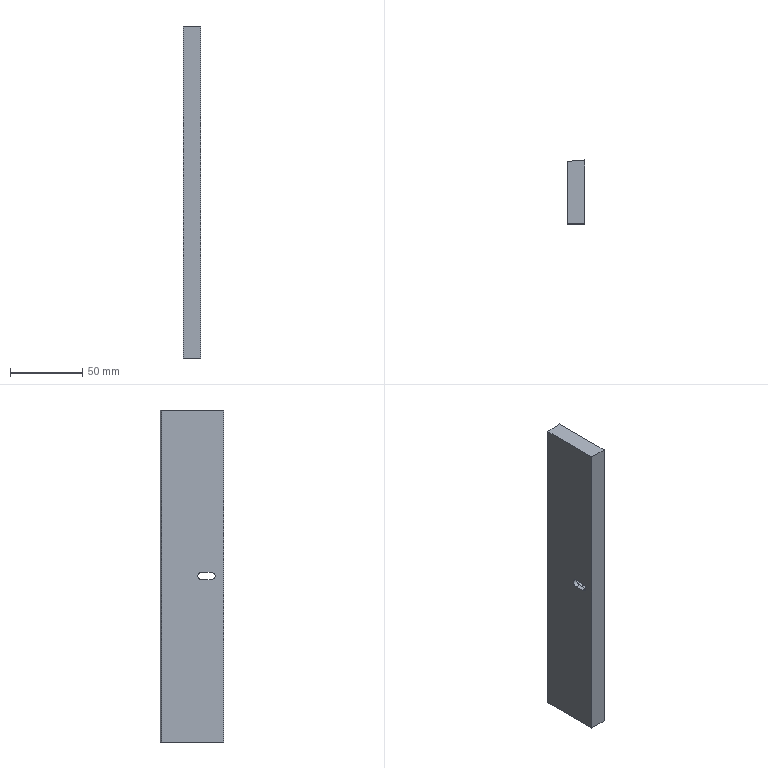Part | STEP file | A14-028 | 1 solid | 15 faces | box 12 x 44 x 230 mm | volume 118590 mm3 | plane 11 | cylinder 4 | commonest cylinder face diameters 5.5 x2 10 x2
STEP:
#1=CARTESIAN_POINT('',(0.,0.,0.));
#2=DIRECTION('',(0.,0.,1.));
#3=DIRECTION('',(1.,0.,0.));
#4=AXIS2_PLACEMENT_3D('',#1,#2,#3);
#5=CARTESIAN_POINT('',(-6.,21.,-115.));
#6=VERTEX_POINT('',#5);
#7=CARTESIAN_POINT('',(-6.,-22.,-115.));
#8=VERTEX_POINT('',#7);
#9=CARTESIAN_POINT('',(-6.,-22.,-115.));
#10=DIRECTION('',(0.,-1.,0.));
#11=VECTOR('',#10,1.);
#12=LINE('',#9,#11);
#13=CARTESIAN_POINT('',(-6.,-22.,115.));
#14=DIRECTION('',(1.,0.,0.));
#15=DIRECTION('',(0.,1.,0.));
#16=AXIS2_PLACEMENT_3D('',#13,#14,#15);
#17=PLANE('',#16);
#18=CARTESIAN_POINT('',(0.,-230.));
#19=DIRECTION('',(-1.,0.));
#20=VECTOR('',#19,1.);
#21=LINE('',#18,#20);
#22=(GEOMETRIC_REPRESENTATION_CONTEXT(2)PARAMETRIC_REPRESENTATION_CONTEXT()REPRESENTATION_CONTEXT('',''));
#23=DEFINITIONAL_REPRESENTATION('',(#21),#22);
#24=PCURVE('',#17,#23);
#25=CARTESIAN_POINT('',(0.,0.,-115.));
#26=DIRECTION('',(0.,0.,1.));
#27=DIRECTION('',(1.,0.,0.));
#28=AXIS2_PLACEMENT_3D('',#25,#26,#27);
#29=PLANE('',#28);
#30=CARTESIAN_POINT('',(-6.,-22.));
#31=DIRECTION('',(0.,-1.));
#32=VECTOR('',#31,1.);
#33=LINE('',#30,#32);
#34=(GEOMETRIC_REPRESENTATION_CONTEXT(2)PARAMETRIC_REPRESENTATION_CONTEXT()REPRESENTATION_CONTEXT('',''));
#35=DEFINITIONAL_REPRESENTATION('',(#33),#34);
#36=PCURVE('',#29,#35);
#37=SURFACE_CURVE('',#12,(#24,#36),.PCURVE_S1.);
#38=EDGE_CURVE('',#6,#8,#37,.T.);
#39=ORIENTED_EDGE('',*,*,#38,.T.);
#40=CARTESIAN_POINT('',(-6.,-22.,115.));
#41=VERTEX_POINT('',#40);
#42=CARTESIAN_POINT('',(-6.,-22.,115.));
#43=DIRECTION('',(0.,0.,-1.));
#44=VECTOR('',#43,1.);
#45=LINE('',#42,#44);
#46=CARTESIAN_POINT('',(0.,0.));
#47=DIRECTION('',(0.,-1.));
#48=VECTOR('',#47,1.);
#49=LINE('',#46,#48);
#50=(GEOMETRIC_REPRESENTATION_CONTEXT(2)PARAMETRIC_REPRESENTATION_CONTEXT()REPRESENTATION_CONTEXT('',''));
#51=DEFINITIONAL_REPRESENTATION('',(#49),#50);
#52=PCURVE('',#17,#51);
#53=CARTESIAN_POINT('',(6.,-22.,115.));
#54=DIRECTION('',(0.,1.,0.));
#55=DIRECTION('',(0.,0.,1.));
#56=AXIS2_PLACEMENT_3D('',#53,#54,#55);
#57=PLANE('',#56);
#58=CARTESIAN_POINT('',(0.,-12.));
#59=DIRECTION('',(-1.,0.));
#60=VECTOR('',#59,1.);
#61=LINE('',#58,#60);
#62=(GEOMETRIC_REPRESENTATION_CONTEXT(2)PARAMETRIC_REPRESENTATION_CONTEXT()REPRESENTATION_CONTEXT('',''));
#63=DEFINITIONAL_REPRESENTATION('',(#61),#62);
#64=PCURVE('',#57,#63);
#65=SURFACE_CURVE('',#45,(#52,#64),.PCURVE_S1.);
#66=EDGE_CURVE('',#41,#8,#65,.T.);
#67=ORIENTED_EDGE('',*,*,#66,.F.);
#68=CARTESIAN_POINT('',(-6.,21.,115.));
#69=VERTEX_POINT('',#68);
#70=CARTESIAN_POINT('',(-6.,-22.,115.));
#71=DIRECTION('',(0.,-1.,0.));
#72=VECTOR('',#71,1.);
#73=LINE('',#70,#72);
#74=CARTESIAN_POINT('',(0.,0.));
#75=DIRECTION('',(-1.,0.));
#76=VECTOR('',#75,1.);
#77=LINE('',#74,#76);
#78=(GEOMETRIC_REPRESENTATION_CONTEXT(2)PARAMETRIC_REPRESENTATION_CONTEXT()REPRESENTATION_CONTEXT('',''));
#79=DEFINITIONAL_REPRESENTATION('',(#77),#78);
#80=PCURVE('',#17,#79);
#81=CARTESIAN_POINT('',(0.,0.,115.));
#82=DIRECTION('',(0.,0.,1.));
#83=DIRECTION('',(1.,0.,0.));
#84=AXIS2_PLACEMENT_3D('',#81,#82,#83);
#85=PLANE('',#84);
#86=CARTESIAN_POINT('',(-6.,-22.));
#87=DIRECTION('',(0.,-1.));
#88=VECTOR('',#87,1.);
#89=LINE('',#86,#88);
#90=(GEOMETRIC_REPRESENTATION_CONTEXT(2)PARAMETRIC_REPRESENTATION_CONTEXT()REPRESENTATION_CONTEXT('',''));
#91=DEFINITIONAL_REPRESENTATION('',(#89),#90);
#92=PCURVE('',#85,#91);
#93=SURFACE_CURVE('',#73,(#80,#92),.PCURVE_S1.);
#94=EDGE_CURVE('',#69,#41,#93,.T.);
#95=ORIENTED_EDGE('',*,*,#94,.F.);
#96=CARTESIAN_POINT('',(-6.,21.,115.));
#97=DIRECTION('',(0.,0.,-1.));
#98=VECTOR('',#97,1.);
#99=LINE('',#96,#98);
#100=CARTESIAN_POINT('',(43.,0.));
#101=DIRECTION('',(0.,-1.));
#102=VECTOR('',#101,1.);
#103=LINE('',#100,#102);
#104=(GEOMETRIC_REPRESENTATION_CONTEXT(2)PARAMETRIC_REPRESENTATION_CONTEXT()REPRESENTATION_CONTEXT('',''));
#105=DEFINITIONAL_REPRESENTATION('',(#103),#104);
#106=PCURVE('',#17,#105);
#107=CARTESIAN_POINT('',(6.,22.,115.));
#108=DIRECTION('',(0.08305,-0.9965,0.));
#109=DIRECTION('',(0.9965,0.08305,0.));
#110=AXIS2_PLACEMENT_3D('',#107,#108,#109);
#111=PLANE('',#110);
#112=CARTESIAN_POINT('',(-12.042,0.));
#113=DIRECTION('',(0.,-1.));
#114=VECTOR('',#113,1.);
#115=LINE('',#112,#114);
#116=(GEOMETRIC_REPRESENTATION_CONTEXT(2)PARAMETRIC_REPRESENTATION_CONTEXT()REPRESENTATION_CONTEXT('',''));
#117=DEFINITIONAL_REPRESENTATION('',(#115),#116);
#118=PCURVE('',#111,#117);
#119=SURFACE_CURVE('',#99,(#106,#118),.PCURVE_S1.);
#120=EDGE_CURVE('',#69,#6,#119,.T.);
#121=ORIENTED_EDGE('',*,*,#120,.T.);
#122=EDGE_LOOP('',(#39,#67,#95,#121));
#123=FACE_BOUND('',#122,.T.);
#124=CARTESIAN_POINT('',(-6.,-13.25,2.75));
#125=VERTEX_POINT('',#124);
#126=CARTESIAN_POINT('',(-6.,-6.75,2.75));
#127=VERTEX_POINT('',#126);
#128=CARTESIAN_POINT('',(-6.,-13.25,2.75));
#129=DIRECTION('',(0.,1.,0.));
#130=VECTOR('',#129,1.);
#131=LINE('',#128,#130);
#132=CARTESIAN_POINT('',(8.75,-112.25));
#133=DIRECTION('',(1.,0.));
#134=VECTOR('',#133,1.);
#135=LINE('',#132,#134);
#136=(GEOMETRIC_REPRESENTATION_CONTEXT(2)PARAMETRIC_REPRESENTATION_CONTEXT()REPRESENTATION_CONTEXT('',''));
#137=DEFINITIONAL_REPRESENTATION('',(#135),#136);
#138=PCURVE('',#17,#137);
#139=CARTESIAN_POINT('',(6.,-13.25,2.75));
#140=DIRECTION('',(0.,0.,1.));
#141=DIRECTION('',(0.,-1.,0.));
#142=AXIS2_PLACEMENT_3D('',#139,#140,#141);
#143=PLANE('',#142);
#144=CARTESIAN_POINT('',(0.,-12.));
#145=DIRECTION('',(-1.,0.));
#146=VECTOR('',#145,1.);
#147=LINE('',#144,#146);
#148=(GEOMETRIC_REPRESENTATION_CONTEXT(2)PARAMETRIC_REPRESENTATION_CONTEXT()REPRESENTATION_CONTEXT('',''));
#149=DEFINITIONAL_REPRESENTATION('',(#147),#148);
#150=PCURVE('',#143,#149);
#151=SURFACE_CURVE('',#131,(#138,#150),.PCURVE_S1.);
#152=EDGE_CURVE('',#125,#127,#151,.T.);
#153=ORIENTED_EDGE('',*,*,#152,.F.);
#154=CARTESIAN_POINT('',(-6.,-13.25,-2.75));
#155=VERTEX_POINT('',#154);
#156=CARTESIAN_POINT('',(-6.,-13.25,0.));
#157=DIRECTION('',(1.,0.,0.));
#158=DIRECTION('',(0.,0.,-1.));
#159=AXIS2_PLACEMENT_3D('',#156,#157,#158);
#160=CIRCLE('',#159,2.75);
#161=CARTESIAN_POINT('',(8.75,-115.));
#162=DIRECTION('',(0.,-1.));
#163=AXIS2_PLACEMENT_2D('',#161,#162);
#164=CIRCLE('',#163,2.75);
#165=(GEOMETRIC_REPRESENTATION_CONTEXT(2)PARAMETRIC_REPRESENTATION_CONTEXT()REPRESENTATION_CONTEXT('',''));
#166=DEFINITIONAL_REPRESENTATION('',(#164),#165);
#167=PCURVE('',#17,#166);
#168=CARTESIAN_POINT('',(6.,-13.25,0.));
#169=DIRECTION('',(1.,0.,0.));
#170=DIRECTION('',(0.,0.,-1.));
#171=AXIS2_PLACEMENT_3D('',#168,#169,#170);
#172=CYLINDRICAL_SURFACE('',#171,2.75);
#173=CARTESIAN_POINT('',(0.,-12.));
#174=DIRECTION('',(1.,0.));
#175=VECTOR('',#174,1.);
#176=LINE('',#173,#175);
#177=(GEOMETRIC_REPRESENTATION_CONTEXT(2)PARAMETRIC_REPRESENTATION_CONTEXT()REPRESENTATION_CONTEXT('',''));
#178=DEFINITIONAL_REPRESENTATION('',(#176),#177);
#179=PCURVE('',#172,#178);
#180=SURFACE_CURVE('',#160,(#167,#179),.PCURVE_S1.);
#181=EDGE_CURVE('',#125,#155,#180,.T.);
#182=ORIENTED_EDGE('',*,*,#181,.T.);
#183=CARTESIAN_POINT('',(-6.,-6.75,-2.75));
#184=VERTEX_POINT('',#183);
#185=CARTESIAN_POINT('',(-6.,-13.25,-2.75));
#186=DIRECTION('',(0.,1.,0.));
#187=VECTOR('',#186,1.);
#188=LINE('',#185,#187);
#189=CARTESIAN_POINT('',(8.75,-117.75));
#190=DIRECTION('',(1.,0.));
#191=VECTOR('',#190,1.);
#192=LINE('',#189,#191);
#193=(GEOMETRIC_REPRESENTATION_CONTEXT(2)PARAMETRIC_REPRESENTATION_CONTEXT()REPRESENTATION_CONTEXT('',''));
#194=DEFINITIONAL_REPRESENTATION('',(#192),#193);
#195=PCURVE('',#17,#194);
#196=CARTESIAN_POINT('',(6.,-13.25,-2.75));
#197=DIRECTION('',(0.,0.,-1.));
#198=DIRECTION('',(0.,1.,0.));
#199=AXIS2_PLACEMENT_3D('',#196,#197,#198);
#200=PLANE('',#199);
#201=CARTESIAN_POINT('',(0.,-12.));
#202=DIRECTION('',(1.,0.));
#203=VECTOR('',#202,1.);
#204=LINE('',#201,#203);
#205=(GEOMETRIC_REPRESENTATION_CONTEXT(2)PARAMETRIC_REPRESENTATION_CONTEXT()REPRESENTATION_CONTEXT('',''));
#206=DEFINITIONAL_REPRESENTATION('',(#204),#205);
#207=PCURVE('',#200,#206);
#208=SURFACE_CURVE('',#188,(#195,#207),.PCURVE_S1.);
#209=EDGE_CURVE('',#155,#184,#208,.T.);
#210=ORIENTED_EDGE('',*,*,#209,.T.);
#211=CARTESIAN_POINT('',(-6.,-6.75,0.));
#212=DIRECTION('',(1.,0.,0.));
#213=DIRECTION('',(0.,0.,-1.));
#214=AXIS2_PLACEMENT_3D('',#211,#212,#213);
#215=CIRCLE('',#214,2.75);
#216=CARTESIAN_POINT('',(15.25,-115.));
#217=DIRECTION('',(0.,-1.));
#218=AXIS2_PLACEMENT_2D('',#216,#217);
#219=CIRCLE('',#218,2.75);
#220=(GEOMETRIC_REPRESENTATION_CONTEXT(2)PARAMETRIC_REPRESENTATION_CONTEXT()REPRESENTATION_CONTEXT('',''));
#221=DEFINITIONAL_REPRESENTATION('',(#219),#220);
#222=PCURVE('',#17,#221);
#223=CARTESIAN_POINT('',(6.,-6.75,0.));
#224=DIRECTION('',(1.,0.,0.));
#225=DIRECTION('',(0.,0.,-1.));
#226=AXIS2_PLACEMENT_3D('',#223,#224,#225);
#227=CYLINDRICAL_SURFACE('',#226,2.75);
#228=CARTESIAN_POINT('',(0.,-12.));
#229=DIRECTION('',(1.,0.));
#230=VECTOR('',#229,1.);
#231=LINE('',#228,#230);
#232=(GEOMETRIC_REPRESENTATION_CONTEXT(2)PARAMETRIC_REPRESENTATION_CONTEXT()REPRESENTATION_CONTEXT('',''));
#233=DEFINITIONAL_REPRESENTATION('',(#231),#232);
#234=PCURVE('',#227,#233);
#235=SURFACE_CURVE('',#215,(#222,#234),.PCURVE_S1.);
#236=EDGE_CURVE('',#184,#127,#235,.T.);
#237=ORIENTED_EDGE('',*,*,#236,.T.);
#238=EDGE_LOOP('',(#153,#182,#210,#237));
#239=FACE_BOUND('',#238,.T.);
#240=ADVANCED_FACE('',(#123,#239),#17,.F.);
#241=CARTESIAN_POINT('',(6.,-13.25,5.));
#242=VERTEX_POINT('',#241);
#243=CARTESIAN_POINT('',(6.,-6.75,5.));
#244=VERTEX_POINT('',#243);
#245=CARTESIAN_POINT('',(6.,-13.25,5.));
#246=DIRECTION('',(0.,1.,0.));
#247=VECTOR('',#246,1.);
#248=LINE('',#245,#247);
#249=CARTESIAN_POINT('',(6.,-22.,115.));
#250=DIRECTION('',(-1.,0.,0.));
#251=DIRECTION('',(0.,-1.,0.));
#252=AXIS2_PLACEMENT_3D('',#249,#250,#251);
#253=PLANE('',#252);
#254=CARTESIAN_POINT('',(-8.75,-110.));
#255=DIRECTION('',(-1.,0.));
#256=VECTOR('',#255,1.);
#257=LINE('',#254,#256);
#258=(GEOMETRIC_REPRESENTATION_CONTEXT(2)PARAMETRIC_REPRESENTATION_CONTEXT()REPRESENTATION_CONTEXT('',''));
#259=DEFINITIONAL_REPRESENTATION('',(#257),#258);
#260=PCURVE('',#253,#259);
#261=CARTESIAN_POINT('',(6.,-13.25,5.));
#262=DIRECTION('',(0.,0.,1.));
#263=DIRECTION('',(0.,-1.,0.));
#264=AXIS2_PLACEMENT_3D('',#261,#262,#263);
#265=PLANE('',#264);
#266=CARTESIAN_POINT('',(0.,0.));
#267=DIRECTION('',(-1.,0.));
#268=VECTOR('',#267,1.);
#269=LINE('',#266,#268);
#270=(GEOMETRIC_REPRESENTATION_CONTEXT(2)PARAMETRIC_REPRESENTATION_CONTEXT()REPRESENTATION_CONTEXT('',''));
#271=DEFINITIONAL_REPRESENTATION('',(#269),#270);
#272=PCURVE('',#265,#271);
#273=SURFACE_CURVE('',#248,(#260,#272),.PCURVE_S1.);
#274=EDGE_CURVE('',#242,#244,#273,.T.);
#275=ORIENTED_EDGE('',*,*,#274,.T.);
#276=CARTESIAN_POINT('',(6.,-6.75,-5.));
#277=VERTEX_POINT('',#276);
#278=CARTESIAN_POINT('',(6.,-6.75,0.));
#279=DIRECTION('',(1.,0.,0.));
#280=DIRECTION('',(0.,0.,-1.));
#281=AXIS2_PLACEMENT_3D('',#278,#279,#280);
#282=CIRCLE('',#281,5.);
#283=CARTESIAN_POINT('',(-15.25,-120.));
#284=CARTESIAN_POINT('',(-23.91,-120.));
#285=CARTESIAN_POINT('',(-19.58,-112.5));
#286=CARTESIAN_POINT('',(-15.25,-105.));
#287=CARTESIAN_POINT('',(-10.92,-112.5));
#288=CARTESIAN_POINT('',(-6.59,-120.));
#289=CARTESIAN_POINT('',(-15.25,-120.));
#290=(BOUNDED_CURVE()B_SPLINE_CURVE(2,(#283,#284,#285,#286,#287,#288,#289),.UNSPECIFIED.,.T.,.F.)B_SPLINE_CURVE_WITH_KNOTS((1,2,2,2,2,1),(-2.094,0.,2.094,4.189,6.283,8.378),.UNSPECIFIED.)CURVE()GEOMETRIC_REPRESENTATION_ITEM()RATIONAL_B_SPLINE_CURVE((1.,0.5,1.,0.5,1.,0.5,1.))REPRESENTATION_ITEM(''));
#291=(GEOMETRIC_REPRESENTATION_CONTEXT(2)PARAMETRIC_REPRESENTATION_CONTEXT()REPRESENTATION_CONTEXT('',''));
#292=DEFINITIONAL_REPRESENTATION('',(#290),#291);
#293=PCURVE('',#253,#292);
#294=CARTESIAN_POINT('',(6.,-6.75,0.));
#295=DIRECTION('',(1.,0.,0.));
#296=DIRECTION('',(0.,0.,-1.));
#297=AXIS2_PLACEMENT_3D('',#294,#295,#296);
#298=CYLINDRICAL_SURFACE('',#297,5.);
#299=CARTESIAN_POINT('',(0.,0.));
#300=DIRECTION('',(1.,0.));
#301=VECTOR('',#300,1.);
#302=LINE('',#299,#301);
#303=(GEOMETRIC_REPRESENTATION_CONTEXT(2)PARAMETRIC_REPRESENTATION_CONTEXT()REPRESENTATION_CONTEXT('',''));
#304=DEFINITIONAL_REPRESENTATION('',(#302),#303);
#305=PCURVE('',#298,#304);
#306=SURFACE_CURVE('',#282,(#293,#305),.PCURVE_S1.);
#307=EDGE_CURVE('',#277,#244,#306,.T.);
#308=ORIENTED_EDGE('',*,*,#307,.F.);
#309=CARTESIAN_POINT('',(6.,-13.25,-5.));
#310=VERTEX_POINT('',#309);
#311=CARTESIAN_POINT('',(6.,-13.25,-5.));
#312=DIRECTION('',(0.,1.,0.));
#313=VECTOR('',#312,1.);
#314=LINE('',#311,#313);
#315=CARTESIAN_POINT('',(-8.75,-120.));
#316=DIRECTION('',(-1.,0.));
#317=VECTOR('',#316,1.);
#318=LINE('',#315,#317);
#319=(GEOMETRIC_REPRESENTATION_CONTEXT(2)PARAMETRIC_REPRESENTATION_CONTEXT()REPRESENTATION_CONTEXT('',''));
#320=DEFINITIONAL_REPRESENTATION('',(#318),#319);
#321=PCURVE('',#253,#320);
#322=CARTESIAN_POINT('',(6.,-13.25,-5.));
#323=DIRECTION('',(0.,0.,-1.));
#324=DIRECTION('',(0.,1.,0.));
#325=AXIS2_PLACEMENT_3D('',#322,#323,#324);
#326=PLANE('',#325);
#327=CARTESIAN_POINT('',(0.,0.));
#328=DIRECTION('',(1.,0.));
#329=VECTOR('',#328,1.);
#330=LINE('',#327,#329);
#331=(GEOMETRIC_REPRESENTATION_CONTEXT(2)PARAMETRIC_REPRESENTATION_CONTEXT()REPRESENTATION_CONTEXT('',''));
#332=DEFINITIONAL_REPRESENTATION('',(#330),#331);
#333=PCURVE('',#326,#332);
#334=SURFACE_CURVE('',#314,(#321,#333),.PCURVE_S1.);
#335=EDGE_CURVE('',#310,#277,#334,.T.);
#336=ORIENTED_EDGE('',*,*,#335,.F.);
#337=CARTESIAN_POINT('',(6.,-13.25,0.));
#338=DIRECTION('',(1.,0.,0.));
#339=DIRECTION('',(0.,0.,-1.));
#340=AXIS2_PLACEMENT_3D('',#337,#338,#339);
#341=CIRCLE('',#340,5.);
#342=CARTESIAN_POINT('',(-8.75,-120.));
#343=CARTESIAN_POINT('',(-17.41,-120.));
#344=CARTESIAN_POINT('',(-13.08,-112.5));
#345=CARTESIAN_POINT('',(-8.75,-105.));
#346=CARTESIAN_POINT('',(-4.42,-112.5));
#347=CARTESIAN_POINT('',(-0.08975,-120.));
#348=CARTESIAN_POINT('',(-8.75,-120.));
#349=(BOUNDED_CURVE()B_SPLINE_CURVE(2,(#342,#343,#344,#345,#346,#347,#348),.UNSPECIFIED.,.T.,.F.)B_SPLINE_CURVE_WITH_KNOTS((1,2,2,2,2,1),(-2.094,0.,2.094,4.189,6.283,8.378),.UNSPECIFIED.)CURVE()GEOMETRIC_REPRESENTATION_ITEM()RATIONAL_B_SPLINE_CURVE((1.,0.5,1.,0.5,1.,0.5,1.))REPRESENTATION_ITEM(''));
#350=(GEOMETRIC_REPRESENTATION_CONTEXT(2)PARAMETRIC_REPRESENTATION_CONTEXT()REPRESENTATION_CONTEXT('',''));
#351=DEFINITIONAL_REPRESENTATION('',(#349),#350);
#352=PCURVE('',#253,#351);
#353=CARTESIAN_POINT('',(6.,-13.25,0.));
#354=DIRECTION('',(1.,0.,0.));
#355=DIRECTION('',(0.,0.,-1.));
#356=AXIS2_PLACEMENT_3D('',#353,#354,#355);
#357=CYLINDRICAL_SURFACE('',#356,5.);
#358=CARTESIAN_POINT('',(0.,0.));
#359=DIRECTION('',(1.,0.));
#360=VECTOR('',#359,1.);
#361=LINE('',#358,#360);
#362=(GEOMETRIC_REPRESENTATION_CONTEXT(2)PARAMETRIC_REPRESENTATION_CONTEXT()REPRESENTATION_CONTEXT('',''));
#363=DEFINITIONAL_REPRESENTATION('',(#361),#362);
#364=PCURVE('',#357,#363);
#365=SURFACE_CURVE('',#341,(#352,#364),.PCURVE_S1.);
#366=EDGE_CURVE('',#242,#310,#365,.T.);
#367=ORIENTED_EDGE('',*,*,#366,.F.);
#368=EDGE_LOOP('',(#275,#308,#336,#367));
#369=FACE_BOUND('',#368,.T.);
#370=CARTESIAN_POINT('',(6.,-22.,-115.));
#371=VERTEX_POINT('',#370);
#372=CARTESIAN_POINT('',(6.,22.,-115.));
#373=VERTEX_POINT('',#372);
#374=CARTESIAN_POINT('',(6.,-22.,-115.));
#375=DIRECTION('',(0.,1.,0.));
#376=VECTOR('',#375,1.);
#377=LINE('',#374,#376);
#378=CARTESIAN_POINT('',(0.,-230.));
#379=DIRECTION('',(-1.,0.));
#380=VECTOR('',#379,1.);
#381=LINE('',#378,#380);
#382=(GEOMETRIC_REPRESENTATION_CONTEXT(2)PARAMETRIC_REPRESENTATION_CONTEXT()REPRESENTATION_CONTEXT('',''));
#383=DEFINITIONAL_REPRESENTATION('',(#381),#382);
#384=PCURVE('',#253,#383);
#385=CARTESIAN_POINT('',(6.,-22.));
#386=DIRECTION('',(0.,1.));
#387=VECTOR('',#386,1.);
#388=LINE('',#385,#387);
#389=(GEOMETRIC_REPRESENTATION_CONTEXT(2)PARAMETRIC_REPRESENTATION_CONTEXT()REPRESENTATION_CONTEXT('',''));
#390=DEFINITIONAL_REPRESENTATION('',(#388),#389);
#391=PCURVE('',#29,#390);
#392=SURFACE_CURVE('',#377,(#384,#391),.PCURVE_S1.);
#393=EDGE_CURVE('',#371,#373,#392,.T.);
#394=ORIENTED_EDGE('',*,*,#393,.T.);
#395=CARTESIAN_POINT('',(6.,22.,115.));
#396=VERTEX_POINT('',#395);
#397=CARTESIAN_POINT('',(6.,22.,115.));
#398=DIRECTION('',(0.,0.,-1.));
#399=VECTOR('',#398,1.);
#400=LINE('',#397,#399);
#401=CARTESIAN_POINT('',(-44.,0.));
#402=DIRECTION('',(0.,-1.));
#403=VECTOR('',#402,1.);
#404=LINE('',#401,#403);
#405=(GEOMETRIC_REPRESENTATION_CONTEXT(2)PARAMETRIC_REPRESENTATION_CONTEXT()REPRESENTATION_CONTEXT('',''));
#406=DEFINITIONAL_REPRESENTATION('',(#404),#405);
#407=PCURVE('',#253,#406);
#408=CARTESIAN_POINT('',(0.,0.));
#409=DIRECTION('',(0.,-1.));
#410=VECTOR('',#409,1.);
#411=LINE('',#408,#410);
#412=(GEOMETRIC_REPRESENTATION_CONTEXT(2)PARAMETRIC_REPRESENTATION_CONTEXT()REPRESENTATION_CONTEXT('',''));
#413=DEFINITIONAL_REPRESENTATION('',(#411),#412);
#414=PCURVE('',#111,#413);
#415=SURFACE_CURVE('',#400,(#407,#414),.PCURVE_S1.);
#416=EDGE_CURVE('',#396,#373,#415,.T.);
#417=ORIENTED_EDGE('',*,*,#416,.F.);
#418=CARTESIAN_POINT('',(6.,-22.,115.));
#419=VERTEX_POINT('',#418);
#420=CARTESIAN_POINT('',(6.,-22.,115.));
#421=DIRECTION('',(0.,1.,0.));
#422=VECTOR('',#421,1.);
#423=LINE('',#420,#422);
#424=CARTESIAN_POINT('',(0.,0.));
#425=DIRECTION('',(-1.,0.));
#426=VECTOR('',#425,1.);
#427=LINE('',#424,#426);
#428=(GEOMETRIC_REPRESENTATION_CONTEXT(2)PARAMETRIC_REPRESENTATION_CONTEXT()REPRESENTATION_CONTEXT('',''));
#429=DEFINITIONAL_REPRESENTATION('',(#427),#428);
#430=PCURVE('',#253,#429);
#431=CARTESIAN_POINT('',(6.,-22.));
#432=DIRECTION('',(0.,1.));
#433=VECTOR('',#432,1.);
#434=LINE('',#431,#433);
#435=(GEOMETRIC_REPRESENTATION_CONTEXT(2)PARAMETRIC_REPRESENTATION_CONTEXT()REPRESENTATION_CONTEXT('',''));
#436=DEFINITIONAL_REPRESENTATION('',(#434),#435);
#437=PCURVE('',#85,#436);
#438=SURFACE_CURVE('',#423,(#430,#437),.PCURVE_S1.);
#439=EDGE_CURVE('',#419,#396,#438,.T.);
#440=ORIENTED_EDGE('',*,*,#439,.F.);
#441=CARTESIAN_POINT('',(6.,-22.,115.));
#442=DIRECTION('',(0.,0.,-1.));
#443=VECTOR('',#442,1.);
#444=LINE('',#441,#443);
#445=CARTESIAN_POINT('',(0.,0.));
#446=DIRECTION('',(0.,-1.));
#447=VECTOR('',#446,1.);
#448=LINE('',#445,#447);
#449=(GEOMETRIC_REPRESENTATION_CONTEXT(2)PARAMETRIC_REPRESENTATION_CONTEXT()REPRESENTATION_CONTEXT('',''));
#450=DEFINITIONAL_REPRESENTATION('',(#448),#449);
#451=PCURVE('',#253,#450);
#452=CARTESIAN_POINT('',(0.,0.));
#453=DIRECTION('',(-1.,0.));
#454=VECTOR('',#453,1.);
#455=LINE('',#452,#454);
#456=(GEOMETRIC_REPRESENTATION_CONTEXT(2)PARAMETRIC_REPRESENTATION_CONTEXT()REPRESENTATION_CONTEXT('',''));
#457=DEFINITIONAL_REPRESENTATION('',(#455),#456);
#458=PCURVE('',#57,#457);
#459=SURFACE_CURVE('',#444,(#451,#458),.PCURVE_S1.);
#460=EDGE_CURVE('',#419,#371,#459,.T.);
#461=ORIENTED_EDGE('',*,*,#460,.T.);
#462=EDGE_LOOP('',(#394,#417,#440,#461));
#463=FACE_BOUND('',#462,.T.);
#464=ADVANCED_FACE('',(#369,#463),#253,.F.);
#465=CARTESIAN_POINT('',(6.,22.,-115.));
#466=DIRECTION('',(-0.9965,-0.08305,0.));
#467=VECTOR('',#466,1.);
#468=LINE('',#465,#467);
#469=CARTESIAN_POINT('',(0.,-230.));
#470=DIRECTION('',(-1.,0.));
#471=VECTOR('',#470,1.);
#472=LINE('',#469,#471);
#473=(GEOMETRIC_REPRESENTATION_CONTEXT(2)PARAMETRIC_REPRESENTATION_CONTEXT()REPRESENTATION_CONTEXT('',''));
#474=DEFINITIONAL_REPRESENTATION('',(#472),#473);
#475=PCURVE('',#111,#474);
#476=CARTESIAN_POINT('',(6.,22.));
#477=DIRECTION('',(-0.9965,-0.08305));
#478=VECTOR('',#477,1.);
#479=LINE('',#476,#478);
#480=(GEOMETRIC_REPRESENTATION_CONTEXT(2)PARAMETRIC_REPRESENTATION_CONTEXT()REPRESENTATION_CONTEXT('',''));
#481=DEFINITIONAL_REPRESENTATION('',(#479),#480);
#482=PCURVE('',#29,#481);
#483=SURFACE_CURVE('',#468,(#475,#482),.PCURVE_S1.);
#484=EDGE_CURVE('',#373,#6,#483,.T.);
#485=ORIENTED_EDGE('',*,*,#484,.T.);
#486=ORIENTED_EDGE('',*,*,#120,.F.);
#487=CARTESIAN_POINT('',(6.,22.,115.));
#488=DIRECTION('',(-0.9965,-0.08305,0.));
#489=VECTOR('',#488,1.);
#490=LINE('',#487,#489);
#491=CARTESIAN_POINT('',(0.,0.));
#492=DIRECTION('',(-1.,0.));
#493=VECTOR('',#492,1.);
#494=LINE('',#491,#493);
#495=(GEOMETRIC_REPRESENTATION_CONTEXT(2)PARAMETRIC_REPRESENTATION_CONTEXT()REPRESENTATION_CONTEXT('',''));
#496=DEFINITIONAL_REPRESENTATION('',(#494),#495);
#497=PCURVE('',#111,#496);
#498=CARTESIAN_POINT('',(6.,22.));
#499=DIRECTION('',(-0.9965,-0.08305));
#500=VECTOR('',#499,1.);
#501=LINE('',#498,#500);
#502=(GEOMETRIC_REPRESENTATION_CONTEXT(2)PARAMETRIC_REPRESENTATION_CONTEXT()REPRESENTATION_CONTEXT('',''));
#503=DEFINITIONAL_REPRESENTATION('',(#501),#502);
#504=PCURVE('',#85,#503);
#505=SURFACE_CURVE('',#490,(#497,#504),.PCURVE_S1.);
#506=EDGE_CURVE('',#396,#69,#505,.T.);
#507=ORIENTED_EDGE('',*,*,#506,.F.);
#508=ORIENTED_EDGE('',*,*,#416,.T.);
#509=EDGE_LOOP('',(#485,#486,#507,#508));
#510=FACE_BOUND('',#509,.T.);
#511=ADVANCED_FACE('',(#510),#111,.F.);
#512=CARTESIAN_POINT('',(6.,-22.,-115.));
#513=DIRECTION('',(1.,0.,0.));
#514=VECTOR('',#513,1.);
#515=LINE('',#512,#514);
#516=CARTESIAN_POINT('',(-230.,0.));
#517=DIRECTION('',(0.,1.));
#518=VECTOR('',#517,1.);
#519=LINE('',#516,#518);
#520=(GEOMETRIC_REPRESENTATION_CONTEXT(2)PARAMETRIC_REPRESENTATION_CONTEXT()REPRESENTATION_CONTEXT('',''));
#521=DEFINITIONAL_REPRESENTATION('',(#519),#520);
#522=PCURVE('',#57,#521);
#523=CARTESIAN_POINT('',(6.,-22.));
#524=DIRECTION('',(1.,0.));
#525=VECTOR('',#524,1.);
#526=LINE('',#523,#525);
#527=(GEOMETRIC_REPRESENTATION_CONTEXT(2)PARAMETRIC_REPRESENTATION_CONTEXT()REPRESENTATION_CONTEXT('',''));
#528=DEFINITIONAL_REPRESENTATION('',(#526),#527);
#529=PCURVE('',#29,#528);
#530=SURFACE_CURVE('',#515,(#522,#529),.PCURVE_S1.);
#531=EDGE_CURVE('',#8,#371,#530,.T.);
#532=ORIENTED_EDGE('',*,*,#531,.T.);
#533=ORIENTED_EDGE('',*,*,#460,.F.);
#534=CARTESIAN_POINT('',(6.,-22.,115.));
#535=DIRECTION('',(1.,0.,0.));
#536=VECTOR('',#535,1.);
#537=LINE('',#534,#536);
#538=CARTESIAN_POINT('',(0.,0.));
#539=DIRECTION('',(0.,1.));
#540=VECTOR('',#539,1.);
#541=LINE('',#538,#540);
#542=(GEOMETRIC_REPRESENTATION_CONTEXT(2)PARAMETRIC_REPRESENTATION_CONTEXT()REPRESENTATION_CONTEXT('',''));
#543=DEFINITIONAL_REPRESENTATION('',(#541),#542);
#544=PCURVE('',#57,#543);
#545=CARTESIAN_POINT('',(6.,-22.));
#546=DIRECTION('',(1.,0.));
#547=VECTOR('',#546,1.);
#548=LINE('',#545,#547);
#549=(GEOMETRIC_REPRESENTATION_CONTEXT(2)PARAMETRIC_REPRESENTATION_CONTEXT()REPRESENTATION_CONTEXT('',''));
#550=DEFINITIONAL_REPRESENTATION('',(#548),#549);
#551=PCURVE('',#85,#550);
#552=SURFACE_CURVE('',#537,(#544,#551),.PCURVE_S1.);
#553=EDGE_CURVE('',#41,#419,#552,.T.);
#554=ORIENTED_EDGE('',*,*,#553,.F.);
#555=ORIENTED_EDGE('',*,*,#66,.T.);
#556=EDGE_LOOP('',(#532,#533,#554,#555));
#557=FACE_BOUND('',#556,.T.);
#558=ADVANCED_FACE('',(#557),#57,.F.);
#559=ORIENTED_EDGE('',*,*,#439,.T.);
#560=ORIENTED_EDGE('',*,*,#506,.T.);
#561=ORIENTED_EDGE('',*,*,#94,.T.);
#562=ORIENTED_EDGE('',*,*,#553,.T.);
#563=EDGE_LOOP('',(#559,#560,#561,#562));
#564=FACE_BOUND('',#563,.T.);
#565=ADVANCED_FACE('',(#564),#85,.T.);
#566=ORIENTED_EDGE('',*,*,#393,.F.);
#567=ORIENTED_EDGE('',*,*,#531,.F.);
#568=ORIENTED_EDGE('',*,*,#38,.F.);
#569=ORIENTED_EDGE('',*,*,#484,.F.);
#570=EDGE_LOOP('',(#566,#567,#568,#569));
#571=FACE_BOUND('',#570,.T.);
#572=ADVANCED_FACE('',(#571),#29,.F.);
#573=CARTESIAN_POINT('',(-3.,-6.75,2.75));
#574=VERTEX_POINT('',#573);
#575=CARTESIAN_POINT('',(6.,-6.75,2.75));
#576=DIRECTION('',(1.,0.,0.));
#577=VECTOR('',#576,1.);
#578=LINE('',#575,#577);
#579=CARTESIAN_POINT('',(3.142,0.));
#580=DIRECTION('',(0.,1.));
#581=VECTOR('',#580,1.);
#582=LINE('',#579,#581);
#583=(GEOMETRIC_REPRESENTATION_CONTEXT(2)PARAMETRIC_REPRESENTATION_CONTEXT()REPRESENTATION_CONTEXT('',''));
#584=DEFINITIONAL_REPRESENTATION('',(#582),#583);
#585=PCURVE('',#227,#584);
#586=CARTESIAN_POINT('',(-6.5,0.));
#587=DIRECTION('',(0.,1.));
#588=VECTOR('',#587,1.);
#589=LINE('',#586,#588);
#590=(GEOMETRIC_REPRESENTATION_CONTEXT(2)PARAMETRIC_REPRESENTATION_CONTEXT()REPRESENTATION_CONTEXT('',''));
#591=DEFINITIONAL_REPRESENTATION('',(#589),#590);
#592=PCURVE('',#143,#591);
#593=SURFACE_CURVE('',#578,(#585,#592),.PCURVE_S1.);
#594=EDGE_CURVE('',#127,#574,#593,.T.);
#595=ORIENTED_EDGE('',*,*,#594,.T.);
#596=CARTESIAN_POINT('',(-3.,-6.75,-2.75));
#597=VERTEX_POINT('',#596);
#598=CARTESIAN_POINT('',(-3.,-6.75,0.));
#599=DIRECTION('',(1.,0.,0.));
#600=DIRECTION('',(0.,0.,-1.));
#601=AXIS2_PLACEMENT_3D('',#598,#599,#600);
#602=CIRCLE('',#601,2.75);
#603=CARTESIAN_POINT('',(0.,-9.));
#604=DIRECTION('',(1.,0.));
#605=VECTOR('',#604,1.);
#606=LINE('',#603,#605);
#607=(GEOMETRIC_REPRESENTATION_CONTEXT(2)PARAMETRIC_REPRESENTATION_CONTEXT()REPRESENTATION_CONTEXT('',''));
#608=DEFINITIONAL_REPRESENTATION('',(#606),#607);
#609=PCURVE('',#227,#608);
#610=CARTESIAN_POINT('',(-3.,-4.,0.));
#611=DIRECTION('',(-1.,0.,0.));
#612=DIRECTION('',(0.,0.,1.));
#613=AXIS2_PLACEMENT_3D('',#610,#611,#612);
#614=PLANE('',#613);
#615=CARTESIAN_POINT('',(-2.75,-2.75));
#616=CARTESIAN_POINT('',(-2.75,2.013));
#617=CARTESIAN_POINT('',(1.375,-0.3684));
#618=CARTESIAN_POINT('',(5.5,-2.75));
#619=CARTESIAN_POINT('',(1.375,-5.132));
#620=CARTESIAN_POINT('',(-2.75,-7.513));
#621=CARTESIAN_POINT('',(-2.75,-2.75));
#622=(BOUNDED_CURVE()B_SPLINE_CURVE(2,(#615,#616,#617,#618,#619,#620,#621),.UNSPECIFIED.,.T.,.F.)B_SPLINE_CURVE_WITH_KNOTS((1,2,2,2,2,1),(-2.094,0.,2.094,4.189,6.283,8.378),.UNSPECIFIED.)CURVE()GEOMETRIC_REPRESENTATION_ITEM()RATIONAL_B_SPLINE_CURVE((1.,0.5,1.,0.5,1.,0.5,1.))REPRESENTATION_ITEM(''));
#623=(GEOMETRIC_REPRESENTATION_CONTEXT(2)PARAMETRIC_REPRESENTATION_CONTEXT()REPRESENTATION_CONTEXT('',''));
#624=DEFINITIONAL_REPRESENTATION('',(#622),#623);
#625=PCURVE('',#614,#624);
#626=SURFACE_CURVE('',#602,(#609,#625),.PCURVE_S1.);
#627=EDGE_CURVE('',#597,#574,#626,.T.);
#628=ORIENTED_EDGE('',*,*,#627,.F.);
#629=CARTESIAN_POINT('',(6.,-6.75,-2.75));
#630=DIRECTION('',(-1.,0.,0.));
#631=VECTOR('',#630,1.);
#632=LINE('',#629,#631);
#633=CARTESIAN_POINT('',(0.,0.));
#634=DIRECTION('',(0.,-1.));
#635=VECTOR('',#634,1.);
#636=LINE('',#633,#635);
#637=(GEOMETRIC_REPRESENTATION_CONTEXT(2)PARAMETRIC_REPRESENTATION_CONTEXT()REPRESENTATION_CONTEXT('',''));
#638=DEFINITIONAL_REPRESENTATION('',(#636),#637);
#639=PCURVE('',#227,#638);
#640=CARTESIAN_POINT('',(6.5,0.));
#641=DIRECTION('',(0.,-1.));
#642=VECTOR('',#641,1.);
#643=LINE('',#640,#642);
#644=(GEOMETRIC_REPRESENTATION_CONTEXT(2)PARAMETRIC_REPRESENTATION_CONTEXT()REPRESENTATION_CONTEXT('',''));
#645=DEFINITIONAL_REPRESENTATION('',(#643),#644);
#646=PCURVE('',#200,#645);
#647=SURFACE_CURVE('',#632,(#639,#646),.PCURVE_S1.);
#648=EDGE_CURVE('',#597,#184,#647,.T.);
#649=ORIENTED_EDGE('',*,*,#648,.T.);
#650=ORIENTED_EDGE('',*,*,#236,.T.);
#651=EDGE_LOOP('',(#595,#628,#649,#650));
#652=FACE_BOUND('',#651,.F.);
#653=ADVANCED_FACE('',(#652),#227,.F.);
#654=CARTESIAN_POINT('',(-3.,-13.25,-2.75));
#655=VERTEX_POINT('',#654);
#656=CARTESIAN_POINT('',(-3.,-13.25,-2.75));
#657=DIRECTION('',(0.,1.,0.));
#658=VECTOR('',#657,1.);
#659=LINE('',#656,#658);
#660=CARTESIAN_POINT('',(-2.75,-9.25));
#661=DIRECTION('',(0.,1.));
#662=VECTOR('',#661,1.);
#663=LINE('',#660,#662);
#664=(GEOMETRIC_REPRESENTATION_CONTEXT(2)PARAMETRIC_REPRESENTATION_CONTEXT()REPRESENTATION_CONTEXT('',''));
#665=DEFINITIONAL_REPRESENTATION('',(#663),#664);
#666=PCURVE('',#614,#665);
#667=CARTESIAN_POINT('',(0.,-9.));
#668=DIRECTION('',(1.,0.));
#669=VECTOR('',#668,1.);
#670=LINE('',#667,#669);
#671=(GEOMETRIC_REPRESENTATION_CONTEXT(2)PARAMETRIC_REPRESENTATION_CONTEXT()REPRESENTATION_CONTEXT('',''));
#672=DEFINITIONAL_REPRESENTATION('',(#670),#671);
#673=PCURVE('',#200,#672);
#674=SURFACE_CURVE('',#659,(#666,#673),.PCURVE_S1.);
#675=EDGE_CURVE('',#655,#597,#674,.T.);
#676=ORIENTED_EDGE('',*,*,#675,.F.);
#677=CARTESIAN_POINT('',(-3.,-13.25,2.75));
#678=VERTEX_POINT('',#677);
#679=CARTESIAN_POINT('',(-3.,-13.25,0.));
#680=DIRECTION('',(1.,0.,0.));
#681=DIRECTION('',(0.,0.,-1.));
#682=AXIS2_PLACEMENT_3D('',#679,#680,#681);
#683=CIRCLE('',#682,2.75);
#684=CARTESIAN_POINT('',(-2.75,-9.25));
#685=CARTESIAN_POINT('',(-2.75,-4.487));
#686=CARTESIAN_POINT('',(1.375,-6.868));
#687=CARTESIAN_POINT('',(5.5,-9.25));
#688=CARTESIAN_POINT('',(1.375,-11.632));
#689=CARTESIAN_POINT('',(-2.75,-14.013));
#690=CARTESIAN_POINT('',(-2.75,-9.25));
#691=(BOUNDED_CURVE()B_SPLINE_CURVE(2,(#684,#685,#686,#687,#688,#689,#690),.UNSPECIFIED.,.T.,.F.)B_SPLINE_CURVE_WITH_KNOTS((1,2,2,2,2,1),(-2.094,0.,2.094,4.189,6.283,8.378),.UNSPECIFIED.)CURVE()GEOMETRIC_REPRESENTATION_ITEM()RATIONAL_B_SPLINE_CURVE((1.,0.5,1.,0.5,1.,0.5,1.))REPRESENTATION_ITEM(''));
#692=(GEOMETRIC_REPRESENTATION_CONTEXT(2)PARAMETRIC_REPRESENTATION_CONTEXT()REPRESENTATION_CONTEXT('',''));
#693=DEFINITIONAL_REPRESENTATION('',(#691),#692);
#694=PCURVE('',#614,#693);
#695=CARTESIAN_POINT('',(0.,-9.));
#696=DIRECTION('',(1.,0.));
#697=VECTOR('',#696,1.);
#698=LINE('',#695,#697);
#699=(GEOMETRIC_REPRESENTATION_CONTEXT(2)PARAMETRIC_REPRESENTATION_CONTEXT()REPRESENTATION_CONTEXT('',''));
#700=DEFINITIONAL_REPRESENTATION('',(#698),#699);
#701=PCURVE('',#172,#700);
#702=SURFACE_CURVE('',#683,(#694,#701),.PCURVE_S1.);
#703=EDGE_CURVE('',#678,#655,#702,.T.);
#704=ORIENTED_EDGE('',*,*,#703,.F.);
#705=CARTESIAN_POINT('',(-3.,-13.25,2.75));
#706=DIRECTION('',(0.,1.,0.));
#707=VECTOR('',#706,1.);
#708=LINE('',#705,#707);
#709=CARTESIAN_POINT('',(2.75,-9.25));
#710=DIRECTION('',(0.,1.));
#711=VECTOR('',#710,1.);
#712=LINE('',#709,#711);
#713=(GEOMETRIC_REPRESENTATION_CONTEXT(2)PARAMETRIC_REPRESENTATION_CONTEXT()REPRESENTATION_CONTEXT('',''));
#714=DEFINITIONAL_REPRESENTATION('',(#712),#713);
#715=PCURVE('',#614,#714);
#716=CARTESIAN_POINT('',(0.,-9.));
#717=DIRECTION('',(-1.,0.));
#718=VECTOR('',#717,1.);
#719=LINE('',#716,#718);
#720=(GEOMETRIC_REPRESENTATION_CONTEXT(2)PARAMETRIC_REPRESENTATION_CONTEXT()REPRESENTATION_CONTEXT('',''));
#721=DEFINITIONAL_REPRESENTATION('',(#719),#720);
#722=PCURVE('',#143,#721);
#723=SURFACE_CURVE('',#708,(#715,#722),.PCURVE_S1.);
#724=EDGE_CURVE('',#678,#574,#723,.T.);
#725=ORIENTED_EDGE('',*,*,#724,.T.);
#726=ORIENTED_EDGE('',*,*,#627,.F.);
#727=EDGE_LOOP('',(#676,#704,#725,#726));
#728=FACE_BOUND('',#727,.T.);
#729=CARTESIAN_POINT('',(-3.,-6.75,-5.));
#730=VERTEX_POINT('',#729);
#731=CARTESIAN_POINT('',(-3.,-6.75,5.));
#732=VERTEX_POINT('',#731);
#733=CARTESIAN_POINT('',(-3.,-6.75,0.));
#734=DIRECTION('',(1.,0.,0.));
#735=DIRECTION('',(0.,0.,-1.));
#736=AXIS2_PLACEMENT_3D('',#733,#734,#735);
#737=CIRCLE('',#736,5.);
#738=CARTESIAN_POINT('',(-5.,-2.75));
#739=CARTESIAN_POINT('',(-5.,5.91));
#740=CARTESIAN_POINT('',(2.5,1.58));
#741=CARTESIAN_POINT('',(10.,-2.75));
#742=CARTESIAN_POINT('',(2.5,-7.08));
#743=CARTESIAN_POINT('',(-5.,-11.41));
#744=CARTESIAN_POINT('',(-5.,-2.75));
#745=(BOUNDED_CURVE()B_SPLINE_CURVE(2,(#738,#739,#740,#741,#742,#743,#744),.UNSPECIFIED.,.T.,.F.)B_SPLINE_CURVE_WITH_KNOTS((1,2,2,2,2,1),(-2.094,0.,2.094,4.189,6.283,8.378),.UNSPECIFIED.)CURVE()GEOMETRIC_REPRESENTATION_ITEM()RATIONAL_B_SPLINE_CURVE((1.,0.5,1.,0.5,1.,0.5,1.))REPRESENTATION_ITEM(''));
#746=(GEOMETRIC_REPRESENTATION_CONTEXT(2)PARAMETRIC_REPRESENTATION_CONTEXT()REPRESENTATION_CONTEXT('',''));
#747=DEFINITIONAL_REPRESENTATION('',(#745),#746);
#748=PCURVE('',#614,#747);
#749=CARTESIAN_POINT('',(0.,-9.));
#750=DIRECTION('',(1.,0.));
#751=VECTOR('',#750,1.);
#752=LINE('',#749,#751);
#753=(GEOMETRIC_REPRESENTATION_CONTEXT(2)PARAMETRIC_REPRESENTATION_CONTEXT()REPRESENTATION_CONTEXT('',''));
#754=DEFINITIONAL_REPRESENTATION('',(#752),#753);
#755=PCURVE('',#298,#754);
#756=SURFACE_CURVE('',#737,(#748,#755),.PCURVE_S1.);
#757=EDGE_CURVE('',#730,#732,#756,.T.);
#758=ORIENTED_EDGE('',*,*,#757,.T.);
#759=CARTESIAN_POINT('',(-3.,-13.25,5.));
#760=VERTEX_POINT('',#759);
#761=CARTESIAN_POINT('',(-3.,-13.25,5.));
#762=DIRECTION('',(0.,1.,0.));
#763=VECTOR('',#762,1.);
#764=LINE('',#761,#763);
#765=CARTESIAN_POINT('',(5.,-9.25));
#766=DIRECTION('',(0.,1.));
#767=VECTOR('',#766,1.);
#768=LINE('',#765,#767);
#769=(GEOMETRIC_REPRESENTATION_CONTEXT(2)PARAMETRIC_REPRESENTATION_CONTEXT()REPRESENTATION_CONTEXT('',''));
#770=DEFINITIONAL_REPRESENTATION('',(#768),#769);
#771=PCURVE('',#614,#770);
#772=CARTESIAN_POINT('',(0.,-9.));
#773=DIRECTION('',(-1.,0.));
#774=VECTOR('',#773,1.);
#775=LINE('',#772,#774);
#776=(GEOMETRIC_REPRESENTATION_CONTEXT(2)PARAMETRIC_REPRESENTATION_CONTEXT()REPRESENTATION_CONTEXT('',''));
#777=DEFINITIONAL_REPRESENTATION('',(#775),#776);
#778=PCURVE('',#265,#777);
#779=SURFACE_CURVE('',#764,(#771,#778),.PCURVE_S1.);
#780=EDGE_CURVE('',#760,#732,#779,.T.);
#781=ORIENTED_EDGE('',*,*,#780,.F.);
#782=CARTESIAN_POINT('',(-3.,-13.25,-5.));
#783=VERTEX_POINT('',#782);
#784=CARTESIAN_POINT('',(-3.,-13.25,0.));
#785=DIRECTION('',(1.,0.,0.));
#786=DIRECTION('',(0.,0.,-1.));
#787=AXIS2_PLACEMENT_3D('',#784,#785,#786);
#788=CIRCLE('',#787,5.);
#789=CARTESIAN_POINT('',(-5.,-9.25));
#790=CARTESIAN_POINT('',(-5.,-0.5897));
#791=CARTESIAN_POINT('',(2.5,-4.92));
#792=CARTESIAN_POINT('',(10.,-9.25));
#793=CARTESIAN_POINT('',(2.5,-13.58));
#794=CARTESIAN_POINT('',(-5.,-17.91));
#795=CARTESIAN_POINT('',(-5.,-9.25));
#796=(BOUNDED_CURVE()B_SPLINE_CURVE(2,(#789,#790,#791,#792,#793,#794,#795),.UNSPECIFIED.,.T.,.F.)B_SPLINE_CURVE_WITH_KNOTS((1,2,2,2,2,1),(-2.094,0.,2.094,4.189,6.283,8.378),.UNSPECIFIED.)CURVE()GEOMETRIC_REPRESENTATION_ITEM()RATIONAL_B_SPLINE_CURVE((1.,0.5,1.,0.5,1.,0.5,1.))REPRESENTATION_ITEM(''));
#797=(GEOMETRIC_REPRESENTATION_CONTEXT(2)PARAMETRIC_REPRESENTATION_CONTEXT()REPRESENTATION_CONTEXT('',''));
#798=DEFINITIONAL_REPRESENTATION('',(#796),#797);
#799=PCURVE('',#614,#798);
#800=CARTESIAN_POINT('',(0.,-9.));
#801=DIRECTION('',(1.,0.));
#802=VECTOR('',#801,1.);
#803=LINE('',#800,#802);
#804=(GEOMETRIC_REPRESENTATION_CONTEXT(2)PARAMETRIC_REPRESENTATION_CONTEXT()REPRESENTATION_CONTEXT('',''));
#805=DEFINITIONAL_REPRESENTATION('',(#803),#804);
#806=PCURVE('',#357,#805);
#807=SURFACE_CURVE('',#788,(#799,#806),.PCURVE_S1.);
#808=EDGE_CURVE('',#760,#783,#807,.T.);
#809=ORIENTED_EDGE('',*,*,#808,.T.);
#810=CARTESIAN_POINT('',(-3.,-13.25,-5.));
#811=DIRECTION('',(0.,1.,0.));
#812=VECTOR('',#811,1.);
#813=LINE('',#810,#812);
#814=CARTESIAN_POINT('',(-5.,-9.25));
#815=DIRECTION('',(0.,1.));
#816=VECTOR('',#815,1.);
#817=LINE('',#814,#816);
#818=(GEOMETRIC_REPRESENTATION_CONTEXT(2)PARAMETRIC_REPRESENTATION_CONTEXT()REPRESENTATION_CONTEXT('',''));
#819=DEFINITIONAL_REPRESENTATION('',(#817),#818);
#820=PCURVE('',#614,#819);
#821=CARTESIAN_POINT('',(0.,-9.));
#822=DIRECTION('',(1.,0.));
#823=VECTOR('',#822,1.);
#824=LINE('',#821,#823);
#825=(GEOMETRIC_REPRESENTATION_CONTEXT(2)PARAMETRIC_REPRESENTATION_CONTEXT()REPRESENTATION_CONTEXT('',''));
#826=DEFINITIONAL_REPRESENTATION('',(#824),#825);
#827=PCURVE('',#326,#826);
#828=SURFACE_CURVE('',#813,(#820,#827),.PCURVE_S1.);
#829=EDGE_CURVE('',#783,#730,#828,.T.);
#830=ORIENTED_EDGE('',*,*,#829,.T.);
#831=EDGE_LOOP('',(#758,#781,#809,#830));
#832=FACE_BOUND('',#831,.T.);
#833=ADVANCED_FACE('',(#728,#832),#614,.F.);
#834=CARTESIAN_POINT('',(6.,-6.75,5.));
#835=DIRECTION('',(1.,0.,0.));
#836=VECTOR('',#835,1.);
#837=LINE('',#834,#836);
#838=CARTESIAN_POINT('',(3.142,0.));
#839=DIRECTION('',(0.,1.));
#840=VECTOR('',#839,1.);
#841=LINE('',#838,#840);
#842=(GEOMETRIC_REPRESENTATION_CONTEXT(2)PARAMETRIC_REPRESENTATION_CONTEXT()REPRESENTATION_CONTEXT('',''));
#843=DEFINITIONAL_REPRESENTATION('',(#841),#842);
#844=PCURVE('',#298,#843);
#845=CARTESIAN_POINT('',(-6.5,0.));
#846=DIRECTION('',(0.,1.));
#847=VECTOR('',#846,1.);
#848=LINE('',#845,#847);
#849=(GEOMETRIC_REPRESENTATION_CONTEXT(2)PARAMETRIC_REPRESENTATION_CONTEXT()REPRESENTATION_CONTEXT('',''));
#850=DEFINITIONAL_REPRESENTATION('',(#848),#849);
#851=PCURVE('',#265,#850);
#852=SURFACE_CURVE('',#837,(#844,#851),.PCURVE_S1.);
#853=EDGE_CURVE('',#732,#244,#852,.T.);
#854=ORIENTED_EDGE('',*,*,#853,.T.);
#855=ORIENTED_EDGE('',*,*,#307,.F.);
#856=CARTESIAN_POINT('',(6.,-6.75,-5.));
#857=DIRECTION('',(-1.,0.,0.));
#858=VECTOR('',#857,1.);
#859=LINE('',#856,#858);
#860=CARTESIAN_POINT('',(0.,0.));
#861=DIRECTION('',(0.,-1.));
#862=VECTOR('',#861,1.);
#863=LINE('',#860,#862);
#864=(GEOMETRIC_REPRESENTATION_CONTEXT(2)PARAMETRIC_REPRESENTATION_CONTEXT()REPRESENTATION_CONTEXT('',''));
#865=DEFINITIONAL_REPRESENTATION('',(#863),#864);
#866=PCURVE('',#298,#865);
#867=CARTESIAN_POINT('',(6.5,0.));
#868=DIRECTION('',(0.,-1.));
#869=VECTOR('',#868,1.);
#870=LINE('',#867,#869);
#871=(GEOMETRIC_REPRESENTATION_CONTEXT(2)PARAMETRIC_REPRESENTATION_CONTEXT()REPRESENTATION_CONTEXT('',''));
#872=DEFINITIONAL_REPRESENTATION('',(#870),#871);
#873=PCURVE('',#326,#872);
#874=SURFACE_CURVE('',#859,(#866,#873),.PCURVE_S1.);
#875=EDGE_CURVE('',#277,#730,#874,.T.);
#876=ORIENTED_EDGE('',*,*,#875,.T.);
#877=ORIENTED_EDGE('',*,*,#757,.T.);
#878=EDGE_LOOP('',(#854,#855,#876,#877));
#879=FACE_BOUND('',#878,.F.);
#880=ADVANCED_FACE('',(#879),#298,.F.);
#881=CARTESIAN_POINT('',(6.,-13.25,2.75));
#882=DIRECTION('',(-1.,0.,0.));
#883=VECTOR('',#882,1.);
#884=LINE('',#881,#883);
#885=CARTESIAN_POINT('',(3.142,0.));
#886=DIRECTION('',(0.,-1.));
#887=VECTOR('',#886,1.);
#888=LINE('',#885,#887);
#889=(GEOMETRIC_REPRESENTATION_CONTEXT(2)PARAMETRIC_REPRESENTATION_CONTEXT()REPRESENTATION_CONTEXT('',''));
#890=DEFINITIONAL_REPRESENTATION('',(#888),#889);
#891=PCURVE('',#172,#890);
#892=CARTESIAN_POINT('',(0.,0.));
#893=DIRECTION('',(0.,-1.));
#894=VECTOR('',#893,1.);
#895=LINE('',#892,#894);
#896=(GEOMETRIC_REPRESENTATION_CONTEXT(2)PARAMETRIC_REPRESENTATION_CONTEXT()REPRESENTATION_CONTEXT('',''));
#897=DEFINITIONAL_REPRESENTATION('',(#895),#896);
#898=PCURVE('',#143,#897);
#899=SURFACE_CURVE('',#884,(#891,#898),.PCURVE_S1.);
#900=EDGE_CURVE('',#678,#125,#899,.T.);
#901=ORIENTED_EDGE('',*,*,#900,.T.);
#902=ORIENTED_EDGE('',*,*,#181,.T.);
#903=CARTESIAN_POINT('',(6.,-13.25,-2.75));
#904=DIRECTION('',(1.,0.,0.));
#905=VECTOR('',#904,1.);
#906=LINE('',#903,#905);
#907=CARTESIAN_POINT('',(6.283,0.));
#908=DIRECTION('',(0.,1.));
#909=VECTOR('',#908,1.);
#910=LINE('',#907,#909);
#911=(GEOMETRIC_REPRESENTATION_CONTEXT(2)PARAMETRIC_REPRESENTATION_CONTEXT()REPRESENTATION_CONTEXT('',''));
#912=DEFINITIONAL_REPRESENTATION('',(#910),#911);
#913=PCURVE('',#172,#912);
#914=CARTESIAN_POINT('',(0.,0.));
#915=DIRECTION('',(0.,1.));
#916=VECTOR('',#915,1.);
#917=LINE('',#914,#916);
#918=(GEOMETRIC_REPRESENTATION_CONTEXT(2)PARAMETRIC_REPRESENTATION_CONTEXT()REPRESENTATION_CONTEXT('',''));
#919=DEFINITIONAL_REPRESENTATION('',(#917),#918);
#920=PCURVE('',#200,#919);
#921=SURFACE_CURVE('',#906,(#913,#920),.PCURVE_S1.);
#922=EDGE_CURVE('',#155,#655,#921,.T.);
#923=ORIENTED_EDGE('',*,*,#922,.T.);
#924=ORIENTED_EDGE('',*,*,#703,.F.);
#925=EDGE_LOOP('',(#901,#902,#923,#924));
#926=FACE_BOUND('',#925,.F.);
#927=ADVANCED_FACE('',(#926),#172,.F.);
#928=CARTESIAN_POINT('',(6.,-13.25,5.));
#929=DIRECTION('',(-1.,0.,0.));
#930=VECTOR('',#929,1.);
#931=LINE('',#928,#930);
#932=CARTESIAN_POINT('',(3.142,0.));
#933=DIRECTION('',(0.,-1.));
#934=VECTOR('',#933,1.);
#935=LINE('',#932,#934);
#936=(GEOMETRIC_REPRESENTATION_CONTEXT(2)PARAMETRIC_REPRESENTATION_CONTEXT()REPRESENTATION_CONTEXT('',''));
#937=DEFINITIONAL_REPRESENTATION('',(#935),#936);
#938=PCURVE('',#357,#937);
#939=CARTESIAN_POINT('',(0.,0.));
#940=DIRECTION('',(0.,-1.));
#941=VECTOR('',#940,1.);
#942=LINE('',#939,#941);
#943=(GEOMETRIC_REPRESENTATION_CONTEXT(2)PARAMETRIC_REPRESENTATION_CONTEXT()REPRESENTATION_CONTEXT('',''));
#944=DEFINITIONAL_REPRESENTATION('',(#942),#943);
#945=PCURVE('',#265,#944);
#946=SURFACE_CURVE('',#931,(#938,#945),.PCURVE_S1.);
#947=EDGE_CURVE('',#242,#760,#946,.T.);
#948=ORIENTED_EDGE('',*,*,#947,.T.);
#949=ORIENTED_EDGE('',*,*,#808,.T.);
#950=CARTESIAN_POINT('',(6.,-13.25,-5.));
#951=DIRECTION('',(1.,0.,0.));
#952=VECTOR('',#951,1.);
#953=LINE('',#950,#952);
#954=CARTESIAN_POINT('',(6.283,0.));
#955=DIRECTION('',(0.,1.));
#956=VECTOR('',#955,1.);
#957=LINE('',#954,#956);
#958=(GEOMETRIC_REPRESENTATION_CONTEXT(2)PARAMETRIC_REPRESENTATION_CONTEXT()REPRESENTATION_CONTEXT('',''));
#959=DEFINITIONAL_REPRESENTATION('',(#957),#958);
#960=PCURVE('',#357,#959);
#961=CARTESIAN_POINT('',(0.,0.));
#962=DIRECTION('',(0.,1.));
#963=VECTOR('',#962,1.);
#964=LINE('',#961,#963);
#965=(GEOMETRIC_REPRESENTATION_CONTEXT(2)PARAMETRIC_REPRESENTATION_CONTEXT()REPRESENTATION_CONTEXT('',''));
#966=DEFINITIONAL_REPRESENTATION('',(#964),#965);
#967=PCURVE('',#326,#966);
#968=SURFACE_CURVE('',#953,(#960,#967),.PCURVE_S1.);
#969=EDGE_CURVE('',#783,#310,#968,.T.);
#970=ORIENTED_EDGE('',*,*,#969,.T.);
#971=ORIENTED_EDGE('',*,*,#366,.F.);
#972=EDGE_LOOP('',(#948,#949,#970,#971));
#973=FACE_BOUND('',#972,.F.);
#974=ADVANCED_FACE('',(#973),#357,.F.);
#975=ORIENTED_EDGE('',*,*,#853,.T.);
#976=ORIENTED_EDGE('',*,*,#274,.F.);
#977=ORIENTED_EDGE('',*,*,#947,.T.);
#978=ORIENTED_EDGE('',*,*,#780,.T.);
#979=EDGE_LOOP('',(#975,#976,#977,#978));
#980=FACE_BOUND('',#979,.T.);
#981=ADVANCED_FACE('',(#980),#265,.F.);
#982=ORIENTED_EDGE('',*,*,#594,.T.);
#983=ORIENTED_EDGE('',*,*,#724,.F.);
#984=ORIENTED_EDGE('',*,*,#900,.T.);
#985=ORIENTED_EDGE('',*,*,#152,.T.);
#986=EDGE_LOOP('',(#982,#983,#984,#985));
#987=FACE_BOUND('',#986,.T.);
#988=ADVANCED_FACE('',(#987),#143,.F.);
#989=ORIENTED_EDGE('',*,*,#648,.T.);
#990=ORIENTED_EDGE('',*,*,#209,.F.);
#991=ORIENTED_EDGE('',*,*,#922,.T.);
#992=ORIENTED_EDGE('',*,*,#675,.T.);
#993=EDGE_LOOP('',(#989,#990,#991,#992));
#994=FACE_BOUND('',#993,.T.);
#995=ADVANCED_FACE('',(#994),#200,.F.);
#996=ORIENTED_EDGE('',*,*,#875,.T.);
#997=ORIENTED_EDGE('',*,*,#829,.F.);
#998=ORIENTED_EDGE('',*,*,#969,.T.);
#999=ORIENTED_EDGE('',*,*,#335,.T.);
#1000=EDGE_LOOP('',(#996,#997,#998,#999));
#1001=FACE_BOUND('',#1000,.T.);
#1002=ADVANCED_FACE('',(#1001),#326,.F.);
#1003=CLOSED_SHELL('',(#240,#464,#511,#558,#565,#572,#653,#833,#880,#927,#974,#981,#988,#995,#1002));
#1004=MANIFOLD_SOLID_BREP('',#1003);
#1005=(LENGTH_UNIT()NAMED_UNIT(*)SI_UNIT(.MILLI.,.METRE.));
#1006=UNCERTAINTY_MEASURE_WITH_UNIT(LENGTH_MEASURE(0.0000001),#1005,'','');
#1007=(NAMED_UNIT(*)PLANE_ANGLE_UNIT()SI_UNIT($,.RADIAN.));
#1008=(NAMED_UNIT(*)SI_UNIT($,.STERADIAN.)SOLID_ANGLE_UNIT());
#1009=(GEOMETRIC_REPRESENTATION_CONTEXT(3)GLOBAL_UNCERTAINTY_ASSIGNED_CONTEXT((#1006))GLOBAL_UNIT_ASSIGNED_CONTEXT((#1005,#1007,#1008))REPRESENTATION_CONTEXT('',''));
#1010=ADVANCED_BREP_SHAPE_REPRESENTATION('',(#4,#1004),#1009);